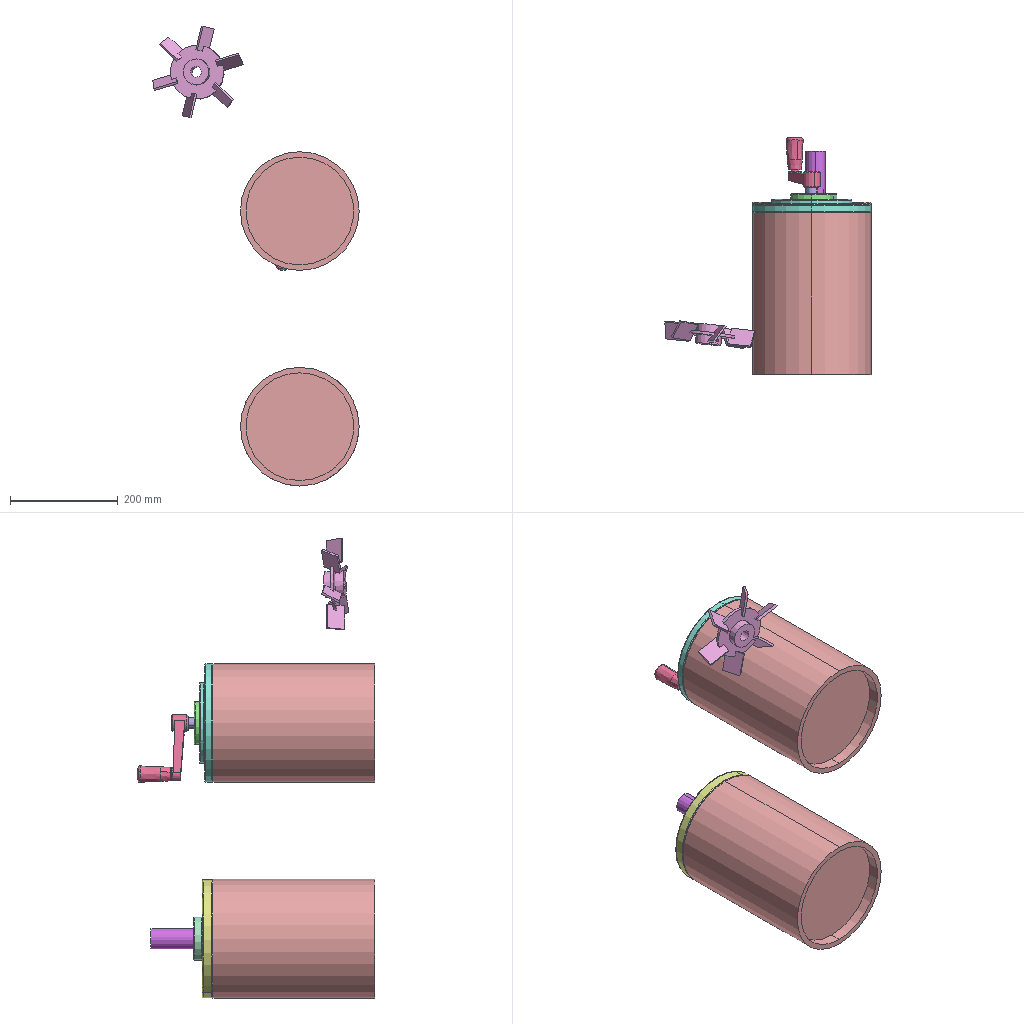Assembly | SolidWorks | 14 different items | 17 placed | box 383 x 440 x 853 mm
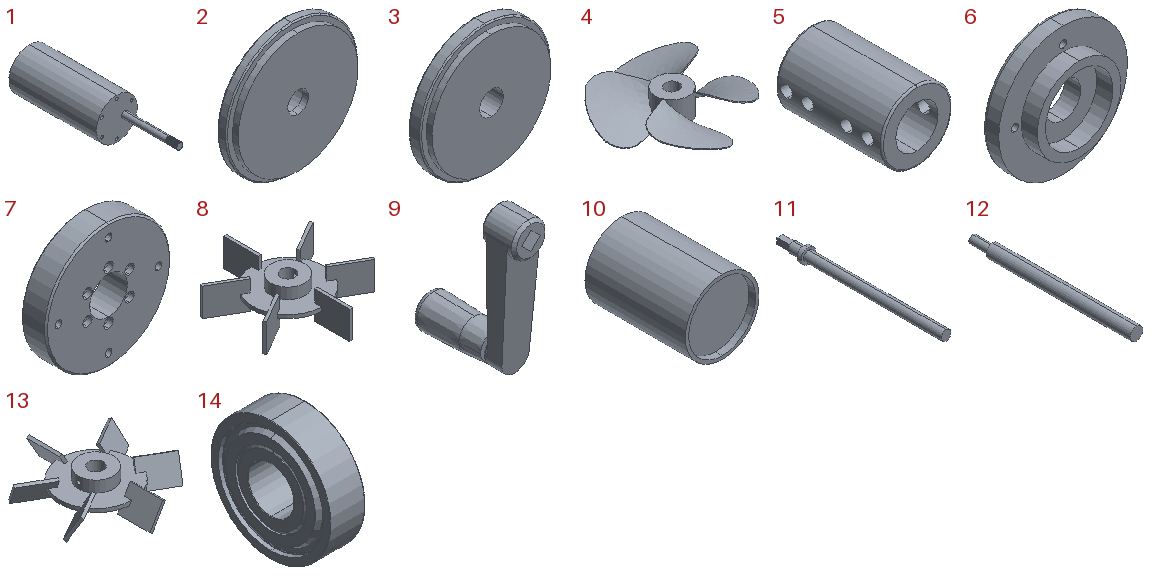Parts list (item | quantity | size | volume | features):
1 | x1 | 37 x 129 x 37 mm | 85867 mm3 | features CirPattern 1, Extrusion 1, HoleWzd 1, ICE 1, SweepThread 1
2 | x1 | 220 x 35 x 220 mm | 996825 mm3 | features ICE 4, Fillet 2, CirPattern 1, Extrusion 1, HoleWzd 1
3 | x1 | 220 x 30 x 220 mm | 1035187 mm3 | features ICE 2, Extrusion 1, Fillet 1, HoleWzd 1, SketchPattern 1
4 | x2 | 178.664 x 178.664 x 37.098 mm | 66695 mm3 | features ICE 2, 3DProfileFeature 1, BaseBody 1, HoleWzd 1, Scale 1
5 | x1 | 20 x 30 x 20 mm | 6976 mm3 | features ICE 2, 3DProfileFeature 1, Extrusion 1, Fillet 1, HoleWzd 1
6 | x1 | 80 x 20 x 80 mm | 52365 mm3 | features ICE 2, CirPattern 1, Extrusion 1, Fillet 1, HoleWzd 1
7 | x1 | 80 x 16 x 80 mm | 70024 mm3 | features HoleWzd 2, Chamfer 1, CirPattern 1, Extrusion 1, SketchPattern 1
8 | x2 | 157.885 x 180 x 40 mm | 130306 mm3 | features ICE 4, 3DProfileFeature 1, BaseBody 1, CirPattern 1, Cut 1, HoleWzd 1, Scale 1
9 | x1 | 31 x 95 x 130.902 mm | 100335 mm3 | features BaseBody 1
10 | x2 | 220 x 300 x 220 mm | 2293363 mm3 | features ICE 2, Extrusion 1
11 | x1 | 30 x 340 x 30 mm | 105361 mm3 | features Cut 1, Extrusion 1, ICE 1
12 | x1 | 20 x 250 x 20 mm | 72508 mm3 | features Cut 1, Extrusion 1
13 | x1 | 157.706 x 170 x 36 mm | 118469 mm3 | features ICE 4, 3DProfileFeature 2, BaseBody 1, CirPattern 1, HoleWzd 1, Scale 1
14 | x1 | 15 x 52 x 52 mm | 22282 mm3 | features BaseBody 1
Mates (type | each side: item.copy, entity, surface, feature):
Coincident | 10.1 plane | assembly plane | 3 times
Concentric | 4.1 face cylinder Input2 | 8.1 face cylinder Input2
Concentric | 10.1 face cylinder Boss-Extrude1 | 2.1 face cylinder Boss-Extrude1
Coincident | 10.1 face plane Boss-Extrude1 | 2.1 face plane Boss-Extrude2
Concentric | 2.1 face cylinder Boss-Extrude2 | 14.1 face cylinder Input1
Coincident | 2.1 face plane Cut-Extrude1 | 14.1 face plane Input1
Concentric | 4.1 face cylinder Cut-Extrude1 | 11.1 face cylinder Boss-Extrude1
Concentric | 2.1 face cylinder Boss-Extrude3 | 6.1 face cylinder Boss-Extrude2
Coincident | 2.1 face plane Boss-Extrude3 | 6.1 face plane Boss-Extrude2
Coincident | 11.1 face plane Cut-Extrude1 | 9.1 face plane Input1 | 3 times
Concentric | 11.1 face cylinder Boss-Extrude1 | 6.1 face cylinder Cut-Extrude1
Concentric | 4.2 face cylinder Input2 | 12.1 face cylinder Boss-Extrude1
Concentric | 10.2 face cylinder Boss-Extrude1 | 3.1 face cylinder Boss-Extrude2
Coincident | 10.2 face plane Boss-Extrude1 | 3.1 face plane Boss-Extrude2
Coincident | 6.1 plane | assembly plane
Parallel | 1.1 plane | assembly plane
Concentric | 12.1 face cylinder Boss-Extrude1 | 1.1 face cylinder Boss-Extrude1
Concentric | 1.1 face cylinder Boss-Extrude2 | 7.1 face cylinder Boss-Extrude1
Coincident | 1.1 face plane Boss-Extrude2 | 7.1 face plane Boss-Extrude1
Coincident | 3.1 face plane Boss-Extrude2 | 7.1 face plane Boss-Extrude1
DistanceDim | 10.2 face plane Boss-Extrude1 | 12.1 face plane Boss-Extrude1
Concentric | 12.1 face cylinder Cut-Extrude1 | 5.1 face cylinder Cut-Extrude2
Coincident | 12.1 face plane Boss-Extrude1 | 5.1 face plane Cut-Extrude2
Parallel | 7.1 plane | assembly plane